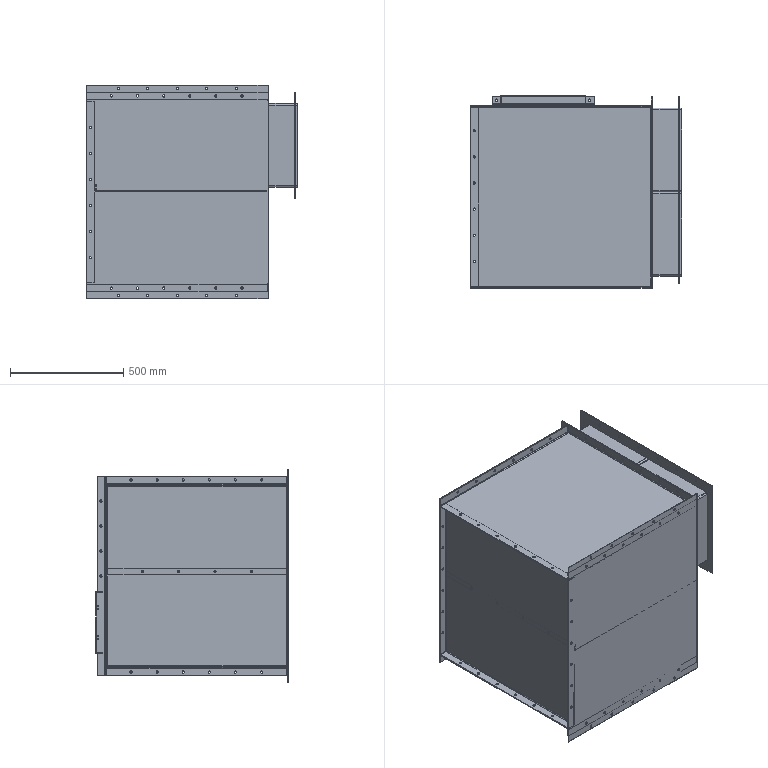Part | SolidWorks | 15 solids | 838 faces | box 930 x 849 x 940 mm | volume 15336660 mm3 | cylinder 558 | plane 254 | spline 26 | commonest cylinder face diameters 10 x444 5 x40 12 x25 6 x21 4.5 x8 8 x8